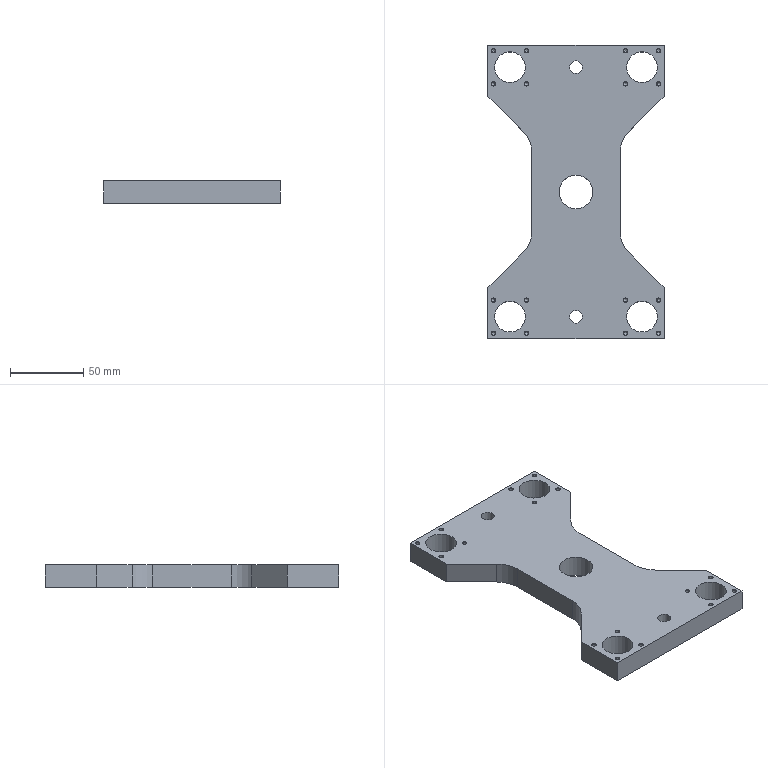Part | STEP file | 冲床-300配套压波_id878_x_t | 1 solid | 73 faces | box 120 x 200 x 15 mm | volume 240910 mm3 | cone 32 | cylinder 27 | plane 14 | commonest cylinder face diameters 2.5 x16 21 x4 40 x4 8.7 x2 23 x1